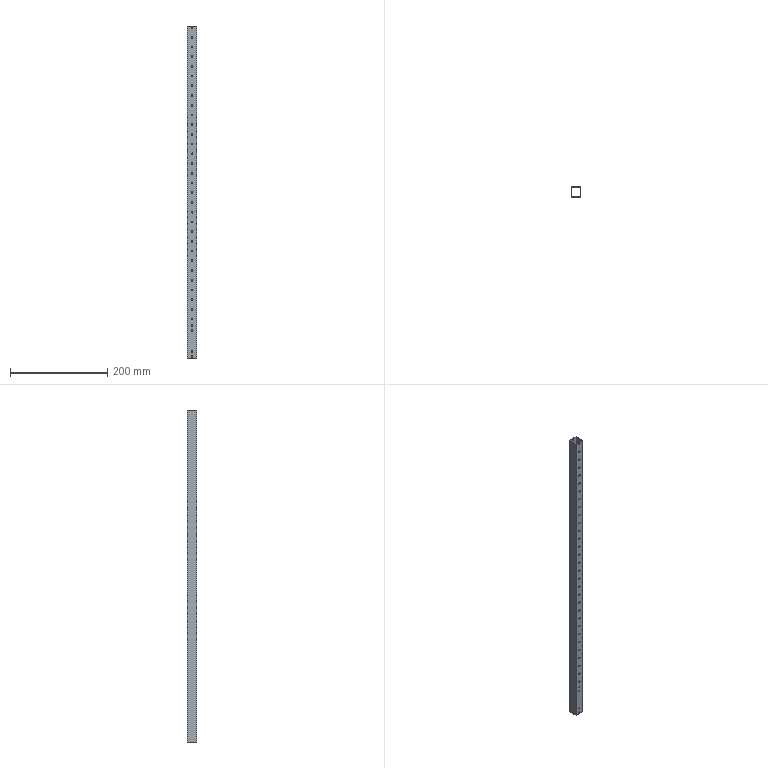Part | SolidWorks | features BaseBody 1 | 1 solid | 150 faces | box 20 x 20 x 683 mm | volume 51247 mm3 | cylinder 140 | plane 10 | commonest cylinder face diameters 3.5 x124 3.2 x16